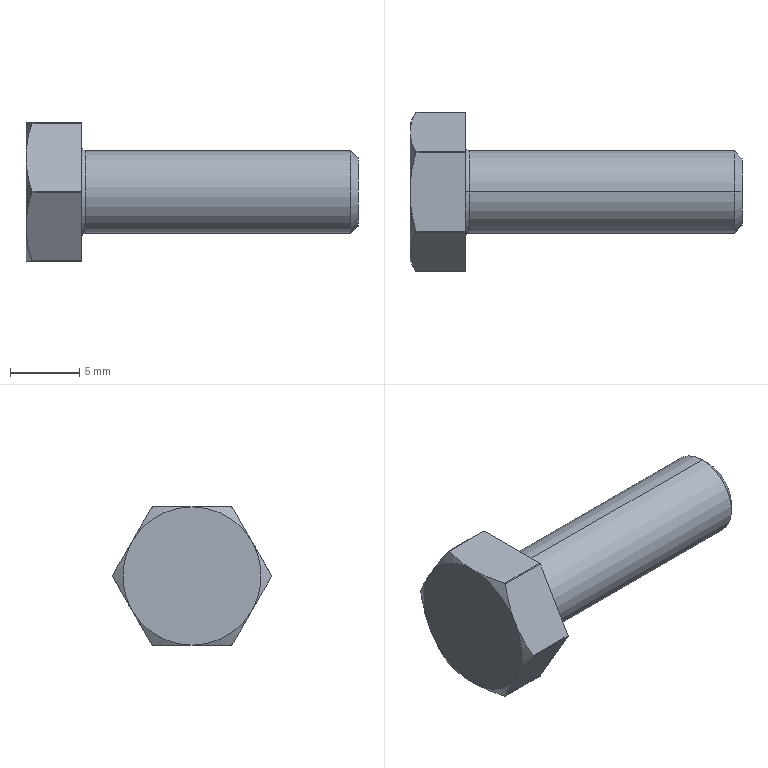Part | STEP file | 11-STRB6-2011_STRB6-20 | 1 solid | 27 faces | box 24 x 11.5 x 10 mm | volume 908.562 mm3 | plane 9 | cylinder 8 | cone 8 | torus 2 | commonest cylinder face diameters 11.5 x6 6 x2
STEP:
#1=CARTESIAN_POINT('',(0.,0.,-3.3));
#2=VERTEX_POINT('',#1);
#3=CARTESIAN_POINT('',(0.,0.,3.3));
#4=VERTEX_POINT('',#3);
#5=CARTESIAN_POINT('',(0.,0.,0.));
#6=DIRECTION('',(-1.,0.,0.));
#7=DIRECTION('',(0.,0.,1.));
#8=AXIS2_PLACEMENT_3D('',#5,#6,#7);
#9=CIRCLE('',#8,3.3);
#10=EDGE_CURVE('',#2,#4,#9,.T.);
#11=ORIENTED_EDGE('',*,*,#10,.F.);
#12=CARTESIAN_POINT('',(0.3,0.,-3.));
#13=VERTEX_POINT('',#12);
#14=CARTESIAN_POINT('',(0.3,0.,-3.3));
#15=DIRECTION('',(0.,1.,0.));
#16=DIRECTION('',(0.,0.,1.));
#17=AXIS2_PLACEMENT_3D('',#14,#15,#16);
#18=CIRCLE('',#17,0.3);
#19=EDGE_CURVE('',#2,#13,#18,.T.);
#20=ORIENTED_EDGE('',*,*,#19,.T.);
#21=CARTESIAN_POINT('',(0.3,0.,3.));
#22=VERTEX_POINT('',#21);
#23=CARTESIAN_POINT('',(0.3,0.,0.));
#24=DIRECTION('',(-1.,0.,0.));
#25=DIRECTION('',(0.,0.,1.));
#26=AXIS2_PLACEMENT_3D('',#23,#24,#25);
#27=CIRCLE('',#26,3.);
#28=EDGE_CURVE('',#13,#22,#27,.T.);
#29=ORIENTED_EDGE('',*,*,#28,.T.);
#30=CARTESIAN_POINT('',(0.3,0.,3.3));
#31=DIRECTION('',(0.,-1.,0.));
#32=DIRECTION('',(0.,0.,-1.));
#33=AXIS2_PLACEMENT_3D('',#30,#31,#32);
#34=CIRCLE('',#33,0.3);
#35=EDGE_CURVE('',#4,#22,#34,.T.);
#36=ORIENTED_EDGE('',*,*,#35,.F.);
#37=EDGE_LOOP('',(#11,#20,#29,#36));
#38=FACE_OUTER_BOUND('',#37,.T.);
#39=CARTESIAN_POINT('',(0.3,0.,0.));
#40=DIRECTION('',(-1.,0.,0.));
#41=DIRECTION('',(0.,0.,1.));
#42=AXIS2_PLACEMENT_3D('',#39,#40,#41);
#43=TOROIDAL_SURFACE('',#42,3.3,0.3);
#44=ADVANCED_FACE('',(#38),#43,.F.);
#45=CARTESIAN_POINT('',(19.459,0.,3.));
#46=VERTEX_POINT('',#45);
#47=CARTESIAN_POINT('',(19.459,0.,-3.));
#48=VERTEX_POINT('',#47);
#49=CARTESIAN_POINT('',(19.459,0.,0.));
#50=DIRECTION('',(-1.,0.,0.));
#51=DIRECTION('',(0.,0.,1.));
#52=AXIS2_PLACEMENT_3D('',#49,#50,#51);
#53=CIRCLE('',#52,3.);
#54=EDGE_CURVE('',#46,#48,#53,.T.);
#55=ORIENTED_EDGE('',*,*,#54,.T.);
#56=CARTESIAN_POINT('',(20.,0.,-3.));
#57=DIRECTION('',(-1.,0.,0.));
#58=VECTOR('',#57,1000.);
#59=LINE('',#56,#58);
#60=EDGE_CURVE('',#48,#13,#59,.T.);
#61=ORIENTED_EDGE('',*,*,#60,.T.);
#62=CARTESIAN_POINT('',(0.3,0.,0.));
#63=DIRECTION('',(-1.,0.,0.));
#64=DIRECTION('',(0.,0.,1.));
#65=AXIS2_PLACEMENT_3D('',#62,#63,#64);
#66=CIRCLE('',#65,3.);
#67=EDGE_CURVE('',#22,#13,#66,.T.);
#68=ORIENTED_EDGE('',*,*,#67,.F.);
#69=CARTESIAN_POINT('',(20.,0.,3.));
#70=DIRECTION('',(-1.,0.,0.));
#71=VECTOR('',#70,1000.);
#72=LINE('',#69,#71);
#73=EDGE_CURVE('',#46,#22,#72,.T.);
#74=ORIENTED_EDGE('',*,*,#73,.F.);
#75=EDGE_LOOP('',(#55,#61,#68,#74));
#76=FACE_OUTER_BOUND('',#75,.T.);
#77=CARTESIAN_POINT('',(20.,0.,0.));
#78=DIRECTION('',(-1.,0.,0.));
#79=DIRECTION('',(0.,0.,1.));
#80=AXIS2_PLACEMENT_3D('',#77,#78,#79);
#81=CYLINDRICAL_SURFACE('',#80,3.);
#82=ADVANCED_FACE('',(#76),#81,.T.);
#83=CARTESIAN_POINT('',(20.,0.,2.458));
#84=VERTEX_POINT('',#83);
#85=CARTESIAN_POINT('',(20.,0.,-2.458));
#86=VERTEX_POINT('',#85);
#87=CARTESIAN_POINT('',(20.,0.,0.));
#88=DIRECTION('',(-1.,0.,0.));
#89=DIRECTION('',(0.,0.,1.));
#90=AXIS2_PLACEMENT_3D('',#87,#88,#89);
#91=CIRCLE('',#90,2.458);
#92=EDGE_CURVE('',#84,#86,#91,.T.);
#93=ORIENTED_EDGE('',*,*,#92,.T.);
#94=CARTESIAN_POINT('',(20.,0.,-2.458));
#95=DIRECTION('',(-0.7071,0.,-0.7071));
#96=VECTOR('',#95,1000.);
#97=LINE('',#94,#96);
#98=EDGE_CURVE('',#86,#48,#97,.T.);
#99=ORIENTED_EDGE('',*,*,#98,.T.);
#100=ORIENTED_EDGE('',*,*,#54,.F.);
#101=CARTESIAN_POINT('',(20.,0.,2.458));
#102=DIRECTION('',(-0.7071,0.,0.7071));
#103=VECTOR('',#102,1000.);
#104=LINE('',#101,#103);
#105=EDGE_CURVE('',#84,#46,#104,.T.);
#106=ORIENTED_EDGE('',*,*,#105,.F.);
#107=EDGE_LOOP('',(#93,#99,#100,#106));
#108=FACE_OUTER_BOUND('',#107,.T.);
#109=CARTESIAN_POINT('',(20.,0.,0.));
#110=DIRECTION('',(-1.,0.,0.));
#111=DIRECTION('',(0.,0.,1.));
#112=AXIS2_PLACEMENT_3D('',#109,#110,#111);
#113=CONICAL_SURFACE('',#112,2.458,0.7854);
#114=ADVANCED_FACE('',(#108),#113,.T.);
#115=CARTESIAN_POINT('',(0.,0.,0.));
#116=DIRECTION('',(-1.,0.,0.));
#117=DIRECTION('',(0.,0.,1.));
#118=AXIS2_PLACEMENT_3D('',#115,#116,#117);
#119=CIRCLE('',#118,3.3);
#120=EDGE_CURVE('',#4,#2,#119,.T.);
#121=ORIENTED_EDGE('',*,*,#120,.T.);
#122=ORIENTED_EDGE('',*,*,#10,.T.);
#123=EDGE_LOOP('',(#121,#122));
#124=FACE_BOUND('',#123,.T.);
#125=CARTESIAN_POINT('',(0.,5.75,0.04096));
#126=VERTEX_POINT('',#125);
#127=CARTESIAN_POINT('',(0.,2.91,4.959));
#128=VERTEX_POINT('',#127);
#129=CARTESIAN_POINT('',(0.,5.774,0.));
#130=DIRECTION('',(0.,-0.5,0.866));
#131=VECTOR('',#130,1000.);
#132=LINE('',#129,#131);
#133=EDGE_CURVE('',#126,#128,#132,.T.);
#134=ORIENTED_EDGE('',*,*,#133,.T.);
#135=CARTESIAN_POINT('',(0.,2.839,5.));
#136=VERTEX_POINT('',#135);
#137=CARTESIAN_POINT('',(0.,0.,0.));
#138=DIRECTION('',(-1.,0.,0.));
#139=DIRECTION('',(0.,0.,1.));
#140=AXIS2_PLACEMENT_3D('',#137,#138,#139);
#141=CIRCLE('',#140,5.75);
#142=EDGE_CURVE('',#136,#128,#141,.T.);
#143=ORIENTED_EDGE('',*,*,#142,.F.);
#144=CARTESIAN_POINT('',(0.,-2.839,5.));
#145=VERTEX_POINT('',#144);
#146=CARTESIAN_POINT('',(0.,2.887,5.));
#147=DIRECTION('',(0.,-1.,0.));
#148=VECTOR('',#147,1000.);
#149=LINE('',#146,#148);
#150=EDGE_CURVE('',#136,#145,#149,.T.);
#151=ORIENTED_EDGE('',*,*,#150,.T.);
#152=CARTESIAN_POINT('',(0.,-2.91,4.959));
#153=VERTEX_POINT('',#152);
#154=CARTESIAN_POINT('',(0.,0.,0.));
#155=DIRECTION('',(-1.,0.,0.));
#156=DIRECTION('',(0.,0.,1.));
#157=AXIS2_PLACEMENT_3D('',#154,#155,#156);
#158=CIRCLE('',#157,5.75);
#159=EDGE_CURVE('',#153,#145,#158,.T.);
#160=ORIENTED_EDGE('',*,*,#159,.F.);
#161=CARTESIAN_POINT('',(0.,-5.75,0.04096));
#162=VERTEX_POINT('',#161);
#163=CARTESIAN_POINT('',(0.,-2.887,5.));
#164=DIRECTION('',(0.,-0.5,-0.866));
#165=VECTOR('',#164,1000.);
#166=LINE('',#163,#165);
#167=EDGE_CURVE('',#153,#162,#166,.T.);
#168=ORIENTED_EDGE('',*,*,#167,.T.);
#169=CARTESIAN_POINT('',(0.,-5.75,-0.04096));
#170=VERTEX_POINT('',#169);
#171=CARTESIAN_POINT('',(0.,0.,0.));
#172=DIRECTION('',(-1.,0.,0.));
#173=DIRECTION('',(0.,0.,1.));
#174=AXIS2_PLACEMENT_3D('',#171,#172,#173);
#175=CIRCLE('',#174,5.75);
#176=EDGE_CURVE('',#170,#162,#175,.T.);
#177=ORIENTED_EDGE('',*,*,#176,.F.);
#178=CARTESIAN_POINT('',(0.,-2.91,-4.959));
#179=VERTEX_POINT('',#178);
#180=CARTESIAN_POINT('',(0.,-5.774,0.));
#181=DIRECTION('',(0.,0.5,-0.866));
#182=VECTOR('',#181,1000.);
#183=LINE('',#180,#182);
#184=EDGE_CURVE('',#170,#179,#183,.T.);
#185=ORIENTED_EDGE('',*,*,#184,.T.);
#186=CARTESIAN_POINT('',(0.,-2.839,-5.));
#187=VERTEX_POINT('',#186);
#188=CARTESIAN_POINT('',(0.,0.,0.));
#189=DIRECTION('',(-1.,0.,0.));
#190=DIRECTION('',(0.,0.,1.));
#191=AXIS2_PLACEMENT_3D('',#188,#189,#190);
#192=CIRCLE('',#191,5.75);
#193=EDGE_CURVE('',#187,#179,#192,.T.);
#194=ORIENTED_EDGE('',*,*,#193,.F.);
#195=CARTESIAN_POINT('',(0.,2.839,-5.));
#196=VERTEX_POINT('',#195);
#197=CARTESIAN_POINT('',(0.,-2.887,-5.));
#198=DIRECTION('',(0.,1.,0.));
#199=VECTOR('',#198,1000.);
#200=LINE('',#197,#199);
#201=EDGE_CURVE('',#187,#196,#200,.T.);
#202=ORIENTED_EDGE('',*,*,#201,.T.);
#203=CARTESIAN_POINT('',(0.,2.91,-4.959));
#204=VERTEX_POINT('',#203);
#205=CARTESIAN_POINT('',(0.,0.,0.));
#206=DIRECTION('',(-1.,0.,0.));
#207=DIRECTION('',(0.,0.,1.));
#208=AXIS2_PLACEMENT_3D('',#205,#206,#207);
#209=CIRCLE('',#208,5.75);
#210=EDGE_CURVE('',#204,#196,#209,.T.);
#211=ORIENTED_EDGE('',*,*,#210,.F.);
#212=CARTESIAN_POINT('',(0.,5.75,-0.04096));
#213=VERTEX_POINT('',#212);
#214=CARTESIAN_POINT('',(0.,2.887,-5.));
#215=DIRECTION('',(0.,0.5,0.866));
#216=VECTOR('',#215,1000.);
#217=LINE('',#214,#216);
#218=EDGE_CURVE('',#204,#213,#217,.T.);
#219=ORIENTED_EDGE('',*,*,#218,.T.);
#220=CARTESIAN_POINT('',(0.,0.,0.));
#221=DIRECTION('',(-1.,0.,0.));
#222=DIRECTION('',(0.,0.,1.));
#223=AXIS2_PLACEMENT_3D('',#220,#221,#222);
#224=CIRCLE('',#223,5.75);
#225=EDGE_CURVE('',#126,#213,#224,.T.);
#226=ORIENTED_EDGE('',*,*,#225,.F.);
#227=EDGE_LOOP('',(#134,#143,#151,#160,#168,#177,#185,#194,#202,#211,#219,#226));
#228=FACE_OUTER_BOUND('',#227,.T.);
#229=CARTESIAN_POINT('',(0.,5.75,0.));
#230=DIRECTION('',(-1.,0.,0.));
#231=DIRECTION('',(0.,0.,1.));
#232=AXIS2_PLACEMENT_3D('',#229,#230,#231);
#233=PLANE('',#232);
#234=ADVANCED_FACE('',(#124,#228),#233,.F.);
#235=CARTESIAN_POINT('',(-3.567,5.75,0.04096));
#236=VERTEX_POINT('',#235);
#237=CARTESIAN_POINT('',(20.,5.75,0.04096));
#238=DIRECTION('',(-1.,0.,0.));
#239=VECTOR('',#238,1000.);
#240=LINE('',#237,#239);
#241=EDGE_CURVE('',#126,#236,#240,.T.);
#242=ORIENTED_EDGE('',*,*,#241,.F.);
#243=ORIENTED_EDGE('',*,*,#225,.T.);
#244=CARTESIAN_POINT('',(-3.567,5.75,-0.04096));
#245=VERTEX_POINT('',#244);
#246=CARTESIAN_POINT('',(20.,5.75,-0.04096));
#247=DIRECTION('',(1.,0.,0.));
#248=VECTOR('',#247,1000.);
#249=LINE('',#246,#248);
#250=EDGE_CURVE('',#245,#213,#249,.T.);
#251=ORIENTED_EDGE('',*,*,#250,.F.);
#252=CARTESIAN_POINT('',(-3.567,0.,0.));
#253=DIRECTION('',(-1.,0.,0.));
#254=DIRECTION('',(0.,0.,1.));
#255=AXIS2_PLACEMENT_3D('',#252,#253,#254);
#256=CIRCLE('',#255,5.75);
#257=EDGE_CURVE('',#236,#245,#256,.T.);
#258=ORIENTED_EDGE('',*,*,#257,.F.);
#259=EDGE_LOOP('',(#242,#243,#251,#258));
#260=FACE_OUTER_BOUND('',#259,.T.);
#261=CARTESIAN_POINT('',(20.,0.,0.));
#262=DIRECTION('',(-1.,0.,0.));
#263=DIRECTION('',(0.,0.,1.));
#264=AXIS2_PLACEMENT_3D('',#261,#262,#263);
#265=CYLINDRICAL_SURFACE('',#264,5.75);
#266=ADVANCED_FACE('',(#260),#265,.T.);
#267=CARTESIAN_POINT('',(-3.567,2.91,4.959));
#268=VERTEX_POINT('',#267);
#269=CARTESIAN_POINT('',(20.,2.91,4.959));
#270=DIRECTION('',(1.,0.,0.));
#271=VECTOR('',#270,1000.);
#272=LINE('',#269,#271);
#273=EDGE_CURVE('',#268,#128,#272,.T.);
#274=ORIENTED_EDGE('',*,*,#273,.F.);
#275=CARTESIAN_POINT('',(-3.567,2.839,5.));
#276=VERTEX_POINT('',#275);
#277=CARTESIAN_POINT('',(-3.567,0.,0.));
#278=DIRECTION('',(-1.,0.,0.));
#279=DIRECTION('',(0.,0.,1.));
#280=AXIS2_PLACEMENT_3D('',#277,#278,#279);
#281=CIRCLE('',#280,5.75);
#282=EDGE_CURVE('',#276,#268,#281,.T.);
#283=ORIENTED_EDGE('',*,*,#282,.F.);
#284=CARTESIAN_POINT('',(20.,2.839,5.));
#285=DIRECTION('',(-1.,0.,0.));
#286=VECTOR('',#285,1000.);
#287=LINE('',#284,#286);
#288=EDGE_CURVE('',#136,#276,#287,.T.);
#289=ORIENTED_EDGE('',*,*,#288,.F.);
#290=ORIENTED_EDGE('',*,*,#142,.T.);
#291=EDGE_LOOP('',(#274,#283,#289,#290));
#292=FACE_OUTER_BOUND('',#291,.T.);
#293=CARTESIAN_POINT('',(20.,0.,0.));
#294=DIRECTION('',(-1.,0.,0.));
#295=DIRECTION('',(0.,0.,1.));
#296=AXIS2_PLACEMENT_3D('',#293,#294,#295);
#297=CYLINDRICAL_SURFACE('',#296,5.75);
#298=ADVANCED_FACE('',(#292),#297,.T.);
#299=CARTESIAN_POINT('',(-3.567,2.91,-4.959));
#300=VERTEX_POINT('',#299);
#301=CARTESIAN_POINT('',(20.,2.91,-4.959));
#302=DIRECTION('',(-1.,0.,0.));
#303=VECTOR('',#302,1000.);
#304=LINE('',#301,#303);
#305=EDGE_CURVE('',#204,#300,#304,.T.);
#306=ORIENTED_EDGE('',*,*,#305,.F.);
#307=ORIENTED_EDGE('',*,*,#210,.T.);
#308=CARTESIAN_POINT('',(-3.567,2.839,-5.));
#309=VERTEX_POINT('',#308);
#310=CARTESIAN_POINT('',(20.,2.839,-5.));
#311=DIRECTION('',(1.,0.,0.));
#312=VECTOR('',#311,1000.);
#313=LINE('',#310,#312);
#314=EDGE_CURVE('',#309,#196,#313,.T.);
#315=ORIENTED_EDGE('',*,*,#314,.F.);
#316=CARTESIAN_POINT('',(-3.567,0.,0.));
#317=DIRECTION('',(-1.,0.,0.));
#318=DIRECTION('',(0.,0.,1.));
#319=AXIS2_PLACEMENT_3D('',#316,#317,#318);
#320=CIRCLE('',#319,5.75);
#321=EDGE_CURVE('',#300,#309,#320,.T.);
#322=ORIENTED_EDGE('',*,*,#321,.F.);
#323=EDGE_LOOP('',(#306,#307,#315,#322));
#324=FACE_OUTER_BOUND('',#323,.T.);
#325=CARTESIAN_POINT('',(20.,0.,0.));
#326=DIRECTION('',(-1.,0.,0.));
#327=DIRECTION('',(0.,0.,1.));
#328=AXIS2_PLACEMENT_3D('',#325,#326,#327);
#329=CYLINDRICAL_SURFACE('',#328,5.75);
#330=ADVANCED_FACE('',(#324),#329,.T.);
#331=CARTESIAN_POINT('',(-3.567,-2.839,-5.));
#332=VERTEX_POINT('',#331);
#333=CARTESIAN_POINT('',(20.,-2.839,-5.));
#334=DIRECTION('',(-1.,0.,0.));
#335=VECTOR('',#334,1000.);
#336=LINE('',#333,#335);
#337=EDGE_CURVE('',#187,#332,#336,.T.);
#338=ORIENTED_EDGE('',*,*,#337,.F.);
#339=ORIENTED_EDGE('',*,*,#193,.T.);
#340=CARTESIAN_POINT('',(-3.567,-2.91,-4.959));
#341=VERTEX_POINT('',#340);
#342=CARTESIAN_POINT('',(20.,-2.91,-4.959));
#343=DIRECTION('',(1.,0.,0.));
#344=VECTOR('',#343,1000.);
#345=LINE('',#342,#344);
#346=EDGE_CURVE('',#341,#179,#345,.T.);
#347=ORIENTED_EDGE('',*,*,#346,.F.);
#348=CARTESIAN_POINT('',(-3.567,0.,0.));
#349=DIRECTION('',(-1.,0.,0.));
#350=DIRECTION('',(0.,0.,1.));
#351=AXIS2_PLACEMENT_3D('',#348,#349,#350);
#352=CIRCLE('',#351,5.75);
#353=EDGE_CURVE('',#332,#341,#352,.T.);
#354=ORIENTED_EDGE('',*,*,#353,.F.);
#355=EDGE_LOOP('',(#338,#339,#347,#354));
#356=FACE_OUTER_BOUND('',#355,.T.);
#357=CARTESIAN_POINT('',(20.,0.,0.));
#358=DIRECTION('',(-1.,0.,0.));
#359=DIRECTION('',(0.,0.,1.));
#360=AXIS2_PLACEMENT_3D('',#357,#358,#359);
#361=CYLINDRICAL_SURFACE('',#360,5.75);
#362=ADVANCED_FACE('',(#356),#361,.T.);
#363=CARTESIAN_POINT('',(-3.567,-5.75,-0.04096));
#364=VERTEX_POINT('',#363);
#365=CARTESIAN_POINT('',(20.,-5.75,-0.04096));
#366=DIRECTION('',(-1.,0.,0.));
#367=VECTOR('',#366,1000.);
#368=LINE('',#365,#367);
#369=EDGE_CURVE('',#170,#364,#368,.T.);
#370=ORIENTED_EDGE('',*,*,#369,.F.);
#371=ORIENTED_EDGE('',*,*,#176,.T.);
#372=CARTESIAN_POINT('',(-3.567,-5.75,0.04096));
#373=VERTEX_POINT('',#372);
#374=CARTESIAN_POINT('',(20.,-5.75,0.04096));
#375=DIRECTION('',(1.,0.,0.));
#376=VECTOR('',#375,1000.);
#377=LINE('',#374,#376);
#378=EDGE_CURVE('',#373,#162,#377,.T.);
#379=ORIENTED_EDGE('',*,*,#378,.F.);
#380=CARTESIAN_POINT('',(-3.567,0.,0.));
#381=DIRECTION('',(-1.,0.,0.));
#382=DIRECTION('',(0.,0.,1.));
#383=AXIS2_PLACEMENT_3D('',#380,#381,#382);
#384=CIRCLE('',#383,5.75);
#385=EDGE_CURVE('',#364,#373,#384,.T.);
#386=ORIENTED_EDGE('',*,*,#385,.F.);
#387=EDGE_LOOP('',(#370,#371,#379,#386));
#388=FACE_OUTER_BOUND('',#387,.T.);
#389=CARTESIAN_POINT('',(20.,0.,0.));
#390=DIRECTION('',(-1.,0.,0.));
#391=DIRECTION('',(0.,0.,1.));
#392=AXIS2_PLACEMENT_3D('',#389,#390,#391);
#393=CYLINDRICAL_SURFACE('',#392,5.75);
#394=ADVANCED_FACE('',(#388),#393,.T.);
#395=CARTESIAN_POINT('',(-3.567,-2.91,4.959));
#396=VERTEX_POINT('',#395);
#397=CARTESIAN_POINT('',(20.,-2.91,4.959));
#398=DIRECTION('',(-1.,0.,0.));
#399=VECTOR('',#398,1000.);
#400=LINE('',#397,#399);
#401=EDGE_CURVE('',#153,#396,#400,.T.);
#402=ORIENTED_EDGE('',*,*,#401,.F.);
#403=ORIENTED_EDGE('',*,*,#159,.T.);
#404=CARTESIAN_POINT('',(-3.567,-2.839,5.));
#405=VERTEX_POINT('',#404);
#406=CARTESIAN_POINT('',(20.,-2.839,5.));
#407=DIRECTION('',(1.,0.,0.));
#408=VECTOR('',#407,1000.);
#409=LINE('',#406,#408);
#410=EDGE_CURVE('',#405,#145,#409,.T.);
#411=ORIENTED_EDGE('',*,*,#410,.F.);
#412=CARTESIAN_POINT('',(-3.567,0.,0.));
#413=DIRECTION('',(-1.,0.,0.));
#414=DIRECTION('',(0.,0.,1.));
#415=AXIS2_PLACEMENT_3D('',#412,#413,#414);
#416=CIRCLE('',#415,5.75);
#417=EDGE_CURVE('',#396,#405,#416,.T.);
#418=ORIENTED_EDGE('',*,*,#417,.F.);
#419=EDGE_LOOP('',(#402,#403,#411,#418));
#420=FACE_OUTER_BOUND('',#419,.T.);
#421=CARTESIAN_POINT('',(20.,0.,0.));
#422=DIRECTION('',(-1.,0.,0.));
#423=DIRECTION('',(0.,0.,1.));
#424=AXIS2_PLACEMENT_3D('',#421,#422,#423);
#425=CYLINDRICAL_SURFACE('',#424,5.75);
#426=ADVANCED_FACE('',(#420),#425,.T.);
#427=CARTESIAN_POINT('',(-4.,4.33,2.5));
#428=VERTEX_POINT('',#427);
#429=CARTESIAN_POINT('',(-3.567,5.75,0.04096));
#430=CARTESIAN_POINT('',(-3.832,5.285,0.8461));
#431=CARTESIAN_POINT('',(-4.,4.813,1.663));
#432=CARTESIAN_POINT('',(-4.,4.33,2.5));
#433=B_SPLINE_CURVE_WITH_KNOTS('',3,(#429,#430,#431,#432),.UNSPECIFIED.,.F.,.F.,(4,4),(0.000000712,0.002873),.UNSPECIFIED.);
#434=EDGE_CURVE('',#236,#428,#433,.T.);
#435=ORIENTED_EDGE('',*,*,#434,.F.);
#436=ORIENTED_EDGE('',*,*,#257,.T.);
#437=CARTESIAN_POINT('',(-4.,4.33,-2.5));
#438=VERTEX_POINT('',#437);
#439=CARTESIAN_POINT('',(-4.,4.33,-2.5));
#440=CARTESIAN_POINT('',(-4.,4.45,-2.292));
#441=CARTESIAN_POINT('',(-3.99,4.571,-2.082));
#442=CARTESIAN_POINT('',(-3.95,4.811,-1.667));
#443=CARTESIAN_POINT('',(-3.921,4.93,-1.461));
#444=CARTESIAN_POINT('',(-3.808,5.284,-0.8471));
#445=CARTESIAN_POINT('',(-3.699,5.518,-0.4424));
#446=CARTESIAN_POINT('',(-3.567,5.75,-0.04096));
#447=B_SPLINE_CURVE_WITH_KNOTS('',3,(#439,#440,#441,#442,#443,#444,#445,#446),.UNSPECIFIED.,.F.,.F.,(4,2,2,4),(0.002873,0.003588,0.004303,0.005733),.UNSPECIFIED.);
#448=EDGE_CURVE('',#438,#245,#447,.T.);
#449=ORIENTED_EDGE('',*,*,#448,.F.);
#450=CARTESIAN_POINT('',(-4.,0.,0.));
#451=DIRECTION('',(-1.,0.,0.));
#452=DIRECTION('',(0.,0.,1.));
#453=AXIS2_PLACEMENT_3D('',#450,#451,#452);
#454=CIRCLE('',#453,5.);
#455=EDGE_CURVE('',#428,#438,#454,.T.);
#456=ORIENTED_EDGE('',*,*,#455,.F.);
#457=EDGE_LOOP('',(#435,#436,#449,#456));
#458=FACE_OUTER_BOUND('',#457,.T.);
#459=CARTESIAN_POINT('',(-3.567,0.,0.));
#460=DIRECTION('',(1.,0.,0.));
#461=DIRECTION('',(0.,0.,-1.));
#462=AXIS2_PLACEMENT_3D('',#459,#460,#461);
#463=CONICAL_SURFACE('',#462,5.75,1.047);
#464=ADVANCED_FACE('',(#458),#463,.T.);
#465=CARTESIAN_POINT('',(-4.,4.33,2.5));
#466=CARTESIAN_POINT('',(-4.,4.21,2.708));
#467=CARTESIAN_POINT('',(-3.99,4.089,2.918));
#468=CARTESIAN_POINT('',(-3.95,3.849,3.333));
#469=CARTESIAN_POINT('',(-3.921,3.73,3.539));
#470=CARTESIAN_POINT('',(-3.808,3.376,4.153));
#471=CARTESIAN_POINT('',(-3.699,3.142,4.558));
#472=CARTESIAN_POINT('',(-3.567,2.91,4.959));
#473=B_SPLINE_CURVE_WITH_KNOTS('',3,(#465,#466,#467,#468,#469,#470,#471,#472),.UNSPECIFIED.,.F.,.F.,(4,2,2,4),(0.002873,0.003588,0.004303,0.005733),.UNSPECIFIED.);
#474=EDGE_CURVE('',#428,#268,#473,.T.);
#475=ORIENTED_EDGE('',*,*,#474,.F.);
#476=CARTESIAN_POINT('',(-4.,0.,5.));
#477=VERTEX_POINT('',#476);
#478=CARTESIAN_POINT('',(-4.,0.,0.));
#479=DIRECTION('',(-1.,0.,0.));
#480=DIRECTION('',(0.,0.,1.));
#481=AXIS2_PLACEMENT_3D('',#478,#479,#480);
#482=CIRCLE('',#481,5.);
#483=EDGE_CURVE('',#477,#428,#482,.T.);
#484=ORIENTED_EDGE('',*,*,#483,.F.);
#485=CARTESIAN_POINT('',(-3.567,2.839,5.));
#486=CARTESIAN_POINT('',(-3.698,2.38,5.));
#487=CARTESIAN_POINT('',(-3.807,1.915,5.));
#488=CARTESIAN_POINT('',(-3.958,0.9662,5.));
#489=CARTESIAN_POINT('',(-4.,0.4799,5.));
#490=CARTESIAN_POINT('',(-4.,0.,5.));
#491=B_SPLINE_CURVE_WITH_KNOTS('',3,(#485,#486,#487,#488,#489,#490),.UNSPECIFIED.,.F.,.F.,(4,2,4),(0.002168,0.0036,0.005033),.UNSPECIFIED.);
#492=EDGE_CURVE('',#276,#477,#491,.T.);
#493=ORIENTED_EDGE('',*,*,#492,.F.);
#494=ORIENTED_EDGE('',*,*,#282,.T.);
#495=EDGE_LOOP('',(#475,#484,#493,#494));
#496=FACE_OUTER_BOUND('',#495,.T.);
#497=CARTESIAN_POINT('',(-3.567,0.,0.));
#498=DIRECTION('',(1.,0.,0.));
#499=DIRECTION('',(0.,0.,-1.));
#500=AXIS2_PLACEMENT_3D('',#497,#498,#499);
#501=CONICAL_SURFACE('',#500,5.75,1.047);
#502=ADVANCED_FACE('',(#496),#501,.T.);
#503=CARTESIAN_POINT('',(-3.567,2.91,-4.959));
#504=CARTESIAN_POINT('',(-3.832,3.375,-4.154));
#505=CARTESIAN_POINT('',(-4.,3.847,-3.337));
#506=CARTESIAN_POINT('',(-4.,4.33,-2.5));
#507=B_SPLINE_CURVE_WITH_KNOTS('',3,(#503,#504,#505,#506),.UNSPECIFIED.,.F.,.F.,(4,4),(0.000000722,0.002873),.UNSPECIFIED.);
#508=EDGE_CURVE('',#300,#438,#507,.T.);
#509=ORIENTED_EDGE('',*,*,#508,.F.);
#510=ORIENTED_EDGE('',*,*,#321,.T.);
#511=CARTESIAN_POINT('',(-4.,0.,-5.));
#512=VERTEX_POINT('',#511);
#513=CARTESIAN_POINT('',(-4.,0.,-5.));
#514=CARTESIAN_POINT('',(-4.,0.4799,-5.));
#515=CARTESIAN_POINT('',(-3.958,0.9662,-5.));
#516=CARTESIAN_POINT('',(-3.807,1.915,-5.));
#517=CARTESIAN_POINT('',(-3.698,2.38,-5.));
#518=CARTESIAN_POINT('',(-3.567,2.839,-5.));
#519=B_SPLINE_CURVE_WITH_KNOTS('',3,(#513,#514,#515,#516,#517,#518),.UNSPECIFIED.,.F.,.F.,(4,2,4),(0.008069,0.009505,0.01094),.UNSPECIFIED.);
#520=EDGE_CURVE('',#512,#309,#519,.T.);
#521=ORIENTED_EDGE('',*,*,#520,.F.);
#522=CARTESIAN_POINT('',(-4.,0.,0.));
#523=DIRECTION('',(-1.,0.,0.));
#524=DIRECTION('',(0.,0.,1.));
#525=AXIS2_PLACEMENT_3D('',#522,#523,#524);
#526=CIRCLE('',#525,5.);
#527=EDGE_CURVE('',#438,#512,#526,.T.);
#528=ORIENTED_EDGE('',*,*,#527,.F.);
#529=EDGE_LOOP('',(#509,#510,#521,#528));
#530=FACE_OUTER_BOUND('',#529,.T.);
#531=CARTESIAN_POINT('',(-3.567,0.,0.));
#532=DIRECTION('',(1.,0.,0.));
#533=DIRECTION('',(0.,0.,-1.));
#534=AXIS2_PLACEMENT_3D('',#531,#532,#533);
#535=CONICAL_SURFACE('',#534,5.75,1.047);
#536=ADVANCED_FACE('',(#530),#535,.T.);
#537=CARTESIAN_POINT('',(-3.567,-2.839,-5.));
#538=CARTESIAN_POINT('',(-3.699,-2.377,-5.));
#539=CARTESIAN_POINT('',(-3.809,-1.904,-5.));
#540=CARTESIAN_POINT('',(-3.959,-0.9562,-5.));
#541=CARTESIAN_POINT('',(-4.,-0.4796,-5.));
#542=CARTESIAN_POINT('',(-4.,0.,-5.));
#543=B_SPLINE_CURVE_WITH_KNOTS('',3,(#537,#538,#539,#540,#541,#542),.UNSPECIFIED.,.F.,.F.,(4,2,4),(0.005197,0.006633,0.008069),.UNSPECIFIED.);
#544=EDGE_CURVE('',#332,#512,#543,.T.);
#545=ORIENTED_EDGE('',*,*,#544,.F.);
#546=ORIENTED_EDGE('',*,*,#353,.T.);
#547=CARTESIAN_POINT('',(-4.,-4.33,-2.5));
#548=VERTEX_POINT('',#547);
#549=CARTESIAN_POINT('',(-4.,-4.33,-2.5));
#550=CARTESIAN_POINT('',(-4.,-4.21,-2.708));
#551=CARTESIAN_POINT('',(-3.99,-4.089,-2.918));
#552=CARTESIAN_POINT('',(-3.95,-3.849,-3.333));
#553=CARTESIAN_POINT('',(-3.921,-3.73,-3.539));
#554=CARTESIAN_POINT('',(-3.808,-3.376,-4.153));
#555=CARTESIAN_POINT('',(-3.699,-3.142,-4.558));
#556=CARTESIAN_POINT('',(-3.567,-2.91,-4.959));
#557=B_SPLINE_CURVE_WITH_KNOTS('',3,(#549,#550,#551,#552,#553,#554,#555,#556),.UNSPECIFIED.,.F.,.F.,(4,2,2,4),(0.002873,0.003588,0.004303,0.005733),.UNSPECIFIED.);
#558=EDGE_CURVE('',#548,#341,#557,.T.);
#559=ORIENTED_EDGE('',*,*,#558,.F.);
#560=CARTESIAN_POINT('',(-4.,0.,0.));
#561=DIRECTION('',(-1.,0.,0.));
#562=DIRECTION('',(0.,0.,1.));
#563=AXIS2_PLACEMENT_3D('',#560,#561,#562);
#564=CIRCLE('',#563,5.);
#565=EDGE_CURVE('',#512,#548,#564,.T.);
#566=ORIENTED_EDGE('',*,*,#565,.F.);
#567=EDGE_LOOP('',(#545,#546,#559,#566));
#568=FACE_OUTER_BOUND('',#567,.T.);
#569=CARTESIAN_POINT('',(-3.567,0.,0.));
#570=DIRECTION('',(1.,0.,0.));
#571=DIRECTION('',(0.,0.,-1.));
#572=AXIS2_PLACEMENT_3D('',#569,#570,#571);
#573=CONICAL_SURFACE('',#572,5.75,1.047);
#574=ADVANCED_FACE('',(#568),#573,.T.);
#575=CARTESIAN_POINT('',(-3.567,-5.75,-0.04096));
#576=CARTESIAN_POINT('',(-3.832,-5.285,-0.8461));
#577=CARTESIAN_POINT('',(-4.,-4.813,-1.663));
#578=CARTESIAN_POINT('',(-4.,-4.33,-2.5));
#579=B_SPLINE_CURVE_WITH_KNOTS('',3,(#575,#576,#577,#578),.UNSPECIFIED.,.F.,.F.,(4,4),(0.000000712,0.002873),.UNSPECIFIED.);
#580=EDGE_CURVE('',#364,#548,#579,.T.);
#581=ORIENTED_EDGE('',*,*,#580,.F.);
#582=ORIENTED_EDGE('',*,*,#385,.T.);
#583=CARTESIAN_POINT('',(-4.,-4.33,2.5));
#584=VERTEX_POINT('',#583);
#585=CARTESIAN_POINT('',(-4.,-4.33,2.5));
#586=CARTESIAN_POINT('',(-4.,-4.45,2.292));
#587=CARTESIAN_POINT('',(-3.99,-4.571,2.082));
#588=CARTESIAN_POINT('',(-3.95,-4.811,1.667));
#589=CARTESIAN_POINT('',(-3.921,-4.93,1.461));
#590=CARTESIAN_POINT('',(-3.808,-5.284,0.8471));
#591=CARTESIAN_POINT('',(-3.699,-5.518,0.4424));
#592=CARTESIAN_POINT('',(-3.567,-5.75,0.04096));
#593=B_SPLINE_CURVE_WITH_KNOTS('',3,(#585,#586,#587,#588,#589,#590,#591,#592),.UNSPECIFIED.,.F.,.F.,(4,2,2,4),(0.002873,0.003588,0.004303,0.005733),.UNSPECIFIED.);
#594=EDGE_CURVE('',#584,#373,#593,.T.);
#595=ORIENTED_EDGE('',*,*,#594,.F.);
#596=CARTESIAN_POINT('',(-4.,0.,0.));
#597=DIRECTION('',(-1.,0.,0.));
#598=DIRECTION('',(0.,0.,1.));
#599=AXIS2_PLACEMENT_3D('',#596,#597,#598);
#600=CIRCLE('',#599,5.);
#601=EDGE_CURVE('',#548,#584,#600,.T.);
#602=ORIENTED_EDGE('',*,*,#601,.F.);
#603=EDGE_LOOP('',(#581,#582,#595,#602));
#604=FACE_OUTER_BOUND('',#603,.T.);
#605=CARTESIAN_POINT('',(-3.567,0.,0.));
#606=DIRECTION('',(1.,0.,0.));
#607=DIRECTION('',(0.,0.,-1.));
#608=AXIS2_PLACEMENT_3D('',#605,#606,#607);
#609=CONICAL_SURFACE('',#608,5.75,1.047);
#610=ADVANCED_FACE('',(#604),#609,.T.);
#611=CARTESIAN_POINT('',(-3.567,-2.91,4.959));
#612=CARTESIAN_POINT('',(-3.832,-3.375,4.154));
#613=CARTESIAN_POINT('',(-4.,-3.847,3.337));
#614=CARTESIAN_POINT('',(-4.,-4.33,2.5));
#615=B_SPLINE_CURVE_WITH_KNOTS('',3,(#611,#612,#613,#614),.UNSPECIFIED.,.F.,.F.,(4,4),(0.000000722,0.002873),.UNSPECIFIED.);
#616=EDGE_CURVE('',#396,#584,#615,.T.);
#617=ORIENTED_EDGE('',*,*,#616,.F.);
#618=ORIENTED_EDGE('',*,*,#417,.T.);
#619=CARTESIAN_POINT('',(-4.,0.,5.));
#620=CARTESIAN_POINT('',(-4.,-0.4796,5.));
#621=CARTESIAN_POINT('',(-3.959,-0.9562,5.));
#622=CARTESIAN_POINT('',(-3.809,-1.904,5.));
#623=CARTESIAN_POINT('',(-3.699,-2.377,5.));
#624=CARTESIAN_POINT('',(-3.567,-2.839,5.));
#625=B_SPLINE_CURVE_WITH_KNOTS('',3,(#619,#620,#621,#622,#623,#624),.UNSPECIFIED.,.F.,.F.,(4,2,4),(0.005033,0.006465,0.007897),.UNSPECIFIED.);
#626=EDGE_CURVE('',#477,#405,#625,.T.);
#627=ORIENTED_EDGE('',*,*,#626,.F.);
#628=CARTESIAN_POINT('',(-4.,0.,0.));
#629=DIRECTION('',(-1.,0.,0.));
#630=DIRECTION('',(0.,0.,1.));
#631=AXIS2_PLACEMENT_3D('',#628,#629,#630);
#632=CIRCLE('',#631,5.);
#633=EDGE_CURVE('',#584,#477,#632,.T.);
#634=ORIENTED_EDGE('',*,*,#633,.F.);
#635=EDGE_LOOP('',(#617,#618,#627,#634));
#636=FACE_OUTER_BOUND('',#635,.T.);
#637=CARTESIAN_POINT('',(-3.567,0.,0.));
#638=DIRECTION('',(1.,0.,0.));
#639=DIRECTION('',(0.,0.,-1.));
#640=AXIS2_PLACEMENT_3D('',#637,#638,#639);
#641=CONICAL_SURFACE('',#640,5.75,1.047);
#642=ADVANCED_FACE('',(#636),#641,.T.);
#643=ORIENTED_EDGE('',*,*,#92,.F.);
#644=CARTESIAN_POINT('',(20.,0.,0.));
#645=DIRECTION('',(-1.,0.,0.));
#646=DIRECTION('',(0.,0.,1.));
#647=AXIS2_PLACEMENT_3D('',#644,#645,#646);
#648=CIRCLE('',#647,2.458);
#649=EDGE_CURVE('',#86,#84,#648,.T.);
#650=ORIENTED_EDGE('',*,*,#649,.F.);
#651=EDGE_LOOP('',(#643,#650));
#652=FACE_OUTER_BOUND('',#651,.T.);
#653=CARTESIAN_POINT('',(20.,2.458,0.));
#654=DIRECTION('',(-1.,0.,0.));
#655=DIRECTION('',(0.,0.,1.));
#656=AXIS2_PLACEMENT_3D('',#653,#654,#655);
#657=PLANE('',#656);
#658=ADVANCED_FACE('',(#652),#657,.F.);
#659=ORIENTED_EDGE('',*,*,#98,.F.);
#660=ORIENTED_EDGE('',*,*,#649,.T.);
#661=ORIENTED_EDGE('',*,*,#105,.T.);
#662=CARTESIAN_POINT('',(19.459,0.,0.));
#663=DIRECTION('',(-1.,0.,0.));
#664=DIRECTION('',(0.,0.,1.));
#665=AXIS2_PLACEMENT_3D('',#662,#663,#664);
#666=CIRCLE('',#665,3.);
#667=EDGE_CURVE('',#48,#46,#666,.T.);
#668=ORIENTED_EDGE('',*,*,#667,.F.);
#669=EDGE_LOOP('',(#659,#660,#661,#668));
#670=FACE_OUTER_BOUND('',#669,.T.);
#671=CARTESIAN_POINT('',(20.,0.,0.));
#672=DIRECTION('',(-1.,0.,0.));
#673=DIRECTION('',(0.,0.,1.));
#674=AXIS2_PLACEMENT_3D('',#671,#672,#673);
#675=CONICAL_SURFACE('',#674,2.458,0.7854);
#676=ADVANCED_FACE('',(#670),#675,.T.);
#677=ORIENTED_EDGE('',*,*,#60,.F.);
#678=ORIENTED_EDGE('',*,*,#667,.T.);
#679=ORIENTED_EDGE('',*,*,#73,.T.);
#680=ORIENTED_EDGE('',*,*,#28,.F.);
#681=EDGE_LOOP('',(#677,#678,#679,#680));
#682=FACE_OUTER_BOUND('',#681,.T.);
#683=CARTESIAN_POINT('',(20.,0.,0.));
#684=DIRECTION('',(-1.,0.,0.));
#685=DIRECTION('',(0.,0.,1.));
#686=AXIS2_PLACEMENT_3D('',#683,#684,#685);
#687=CYLINDRICAL_SURFACE('',#686,3.);
#688=ADVANCED_FACE('',(#682),#687,.T.);
#689=ORIENTED_EDGE('',*,*,#19,.F.);
#690=ORIENTED_EDGE('',*,*,#120,.F.);
#691=ORIENTED_EDGE('',*,*,#35,.T.);
#692=ORIENTED_EDGE('',*,*,#67,.T.);
#693=EDGE_LOOP('',(#689,#690,#691,#692));
#694=FACE_OUTER_BOUND('',#693,.T.);
#695=CARTESIAN_POINT('',(0.3,0.,0.));
#696=DIRECTION('',(-1.,0.,0.));
#697=DIRECTION('',(0.,0.,1.));
#698=AXIS2_PLACEMENT_3D('',#695,#696,#697);
#699=TOROIDAL_SURFACE('',#698,3.3,0.3);
#700=ADVANCED_FACE('',(#694),#699,.F.);
#701=ORIENTED_EDGE('',*,*,#483,.T.);
#702=ORIENTED_EDGE('',*,*,#455,.T.);
#703=ORIENTED_EDGE('',*,*,#527,.T.);
#704=ORIENTED_EDGE('',*,*,#565,.T.);
#705=ORIENTED_EDGE('',*,*,#601,.T.);
#706=ORIENTED_EDGE('',*,*,#633,.T.);
#707=EDGE_LOOP('',(#701,#702,#703,#704,#705,#706));
#708=FACE_OUTER_BOUND('',#707,.T.);
#709=CARTESIAN_POINT('',(-4.,0.,0.));
#710=DIRECTION('',(1.,0.,0.));
#711=DIRECTION('',(0.,0.,-1.));
#712=AXIS2_PLACEMENT_3D('',#709,#710,#711);
#713=PLANE('',#712);
#714=ADVANCED_FACE('',(#708),#713,.F.);
#715=ORIENTED_EDGE('',*,*,#288,.T.);
#716=ORIENTED_EDGE('',*,*,#492,.T.);
#717=ORIENTED_EDGE('',*,*,#626,.T.);
#718=ORIENTED_EDGE('',*,*,#410,.T.);
#719=ORIENTED_EDGE('',*,*,#150,.F.);
#720=EDGE_LOOP('',(#715,#716,#717,#718,#719));
#721=FACE_OUTER_BOUND('',#720,.T.);
#722=CARTESIAN_POINT('',(-4.,2.887,5.));
#723=DIRECTION('',(0.,0.,1.));
#724=DIRECTION('',(1.,0.,0.));
#725=AXIS2_PLACEMENT_3D('',#722,#723,#724);
#726=PLANE('',#725);
#727=ADVANCED_FACE('',(#721),#726,.T.);
#728=ORIENTED_EDGE('',*,*,#401,.T.);
#729=ORIENTED_EDGE('',*,*,#616,.T.);
#730=ORIENTED_EDGE('',*,*,#594,.T.);
#731=ORIENTED_EDGE('',*,*,#378,.T.);
#732=ORIENTED_EDGE('',*,*,#167,.F.);
#733=EDGE_LOOP('',(#728,#729,#730,#731,#732));
#734=FACE_OUTER_BOUND('',#733,.T.);
#735=CARTESIAN_POINT('',(-4.,-2.887,5.));
#736=DIRECTION('',(0.,-0.866,0.5));
#737=DIRECTION('',(0.,-0.5,-0.866));
#738=AXIS2_PLACEMENT_3D('',#735,#736,#737);
#739=PLANE('',#738);
#740=ADVANCED_FACE('',(#734),#739,.T.);
#741=ORIENTED_EDGE('',*,*,#369,.T.);
#742=ORIENTED_EDGE('',*,*,#580,.T.);
#743=ORIENTED_EDGE('',*,*,#558,.T.);
#744=ORIENTED_EDGE('',*,*,#346,.T.);
#745=ORIENTED_EDGE('',*,*,#184,.F.);
#746=EDGE_LOOP('',(#741,#742,#743,#744,#745));
#747=FACE_OUTER_BOUND('',#746,.T.);
#748=CARTESIAN_POINT('',(-4.,-5.774,0.));
#749=DIRECTION('',(0.,-0.866,-0.5));
#750=DIRECTION('',(0.,0.5,-0.866));
#751=AXIS2_PLACEMENT_3D('',#748,#749,#750);
#752=PLANE('',#751);
#753=ADVANCED_FACE('',(#747),#752,.T.);
#754=ORIENTED_EDGE('',*,*,#337,.T.);
#755=ORIENTED_EDGE('',*,*,#544,.T.);
#756=ORIENTED_EDGE('',*,*,#520,.T.);
#757=ORIENTED_EDGE('',*,*,#314,.T.);
#758=ORIENTED_EDGE('',*,*,#201,.F.);
#759=EDGE_LOOP('',(#754,#755,#756,#757,#758));
#760=FACE_OUTER_BOUND('',#759,.T.);
#761=CARTESIAN_POINT('',(-4.,-2.887,-5.));
#762=DIRECTION('',(0.,0.,-1.));
#763=DIRECTION('',(-1.,0.,0.));
#764=AXIS2_PLACEMENT_3D('',#761,#762,#763);
#765=PLANE('',#764);
#766=ADVANCED_FACE('',(#760),#765,.T.);
#767=ORIENTED_EDGE('',*,*,#305,.T.);
#768=ORIENTED_EDGE('',*,*,#508,.T.);
#769=ORIENTED_EDGE('',*,*,#448,.T.);
#770=ORIENTED_EDGE('',*,*,#250,.T.);
#771=ORIENTED_EDGE('',*,*,#218,.F.);
#772=EDGE_LOOP('',(#767,#768,#769,#770,#771));
#773=FACE_OUTER_BOUND('',#772,.T.);
#774=CARTESIAN_POINT('',(-4.,2.887,-5.));
#775=DIRECTION('',(0.,0.866,-0.5));
#776=DIRECTION('',(0.,0.5,0.866));
#777=AXIS2_PLACEMENT_3D('',#774,#775,#776);
#778=PLANE('',#777);
#779=ADVANCED_FACE('',(#773),#778,.T.);
#780=ORIENTED_EDGE('',*,*,#241,.T.);
#781=ORIENTED_EDGE('',*,*,#434,.T.);
#782=ORIENTED_EDGE('',*,*,#474,.T.);
#783=ORIENTED_EDGE('',*,*,#273,.T.);
#784=ORIENTED_EDGE('',*,*,#133,.F.);
#785=EDGE_LOOP('',(#780,#781,#782,#783,#784));
#786=FACE_OUTER_BOUND('',#785,.T.);
#787=CARTESIAN_POINT('',(-4.,5.774,0.));
#788=DIRECTION('',(0.,0.866,0.5));
#789=DIRECTION('',(0.,-0.5,0.866));
#790=AXIS2_PLACEMENT_3D('',#787,#788,#789);
#791=PLANE('',#790);
#792=ADVANCED_FACE('',(#786),#791,.T.);
#793=CLOSED_SHELL('',(#44,#82,#114,#234,#266,#298,#330,#362,#394,#426,#464,#502,#536,#574,#610,#642,#658,#676,#688,#700,#714,#727,#740,#753,#766,#779,#792));
#794=MANIFOLD_SOLID_BREP('',#793);
#795=CARTESIAN_POINT('',(0.,0.,0.));
#796=DIRECTION('',(0.,0.,1.));
#797=DIRECTION('',(1.,0.,0.));
#798=AXIS2_PLACEMENT_3D('',#795,#796,#797);
#799=(LENGTH_UNIT()NAMED_UNIT(*)SI_UNIT(.MILLI.,.METRE.));
#800=UNCERTAINTY_MEASURE_WITH_UNIT(LENGTH_MEASURE(0.00001),#799,'','');
#801=(NAMED_UNIT(*)PLANE_ANGLE_UNIT()SI_UNIT($,.RADIAN.));
#802=(NAMED_UNIT(*)SI_UNIT($,.STERADIAN.)SOLID_ANGLE_UNIT());
#803=(GEOMETRIC_REPRESENTATION_CONTEXT(3)GLOBAL_UNCERTAINTY_ASSIGNED_CONTEXT((#800))GLOBAL_UNIT_ASSIGNED_CONTEXT((#799,#801,#802))REPRESENTATION_CONTEXT('',''));
#804=ADVANCED_BREP_SHAPE_REPRESENTATION('',(#794,#798),#803);